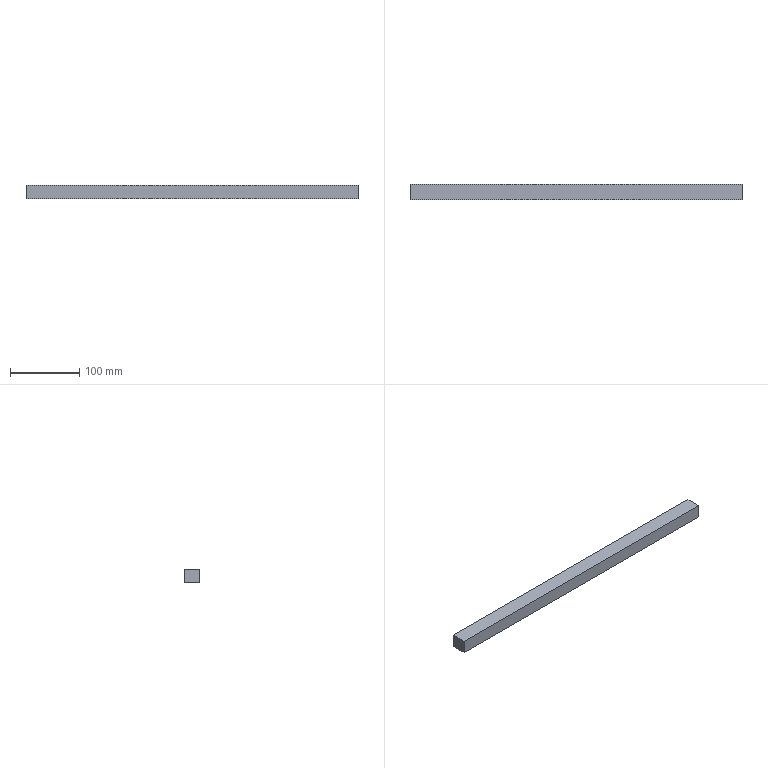Part | SolidWorks | features Extrusion 1 | 1 solid | 6 faces | box 480 x 22 x 20 mm | volume 211200 mm3 | plane 6
STEP:
#1=CARTESIAN_POINT('',(0.,22.,0.));
#2=VERTEX_POINT('',#1);
#3=CARTESIAN_POINT('',(0.,0.,0.));
#4=VERTEX_POINT('',#3);
#5=CARTESIAN_POINT('',(0.,0.,0.));
#6=DIRECTION('',(0.,-1.,0.));
#7=VECTOR('',#6,1000.);
#8=LINE('',#5,#7);
#9=EDGE_CURVE('',#2,#4,#8,.T.);
#10=ORIENTED_EDGE('',*,*,#9,.T.);
#11=CARTESIAN_POINT('',(0.,0.,20.));
#12=VERTEX_POINT('',#11);
#13=CARTESIAN_POINT('',(0.,0.,20.));
#14=DIRECTION('',(0.,0.,-1.));
#15=VECTOR('',#14,1000.);
#16=LINE('',#13,#15);
#17=EDGE_CURVE('',#12,#4,#16,.T.);
#18=ORIENTED_EDGE('',*,*,#17,.F.);
#19=CARTESIAN_POINT('',(0.,22.,20.));
#20=VERTEX_POINT('',#19);
#21=CARTESIAN_POINT('',(0.,0.,20.));
#22=DIRECTION('',(0.,-1.,0.));
#23=VECTOR('',#22,1000.);
#24=LINE('',#21,#23);
#25=EDGE_CURVE('',#20,#12,#24,.T.);
#26=ORIENTED_EDGE('',*,*,#25,.F.);
#27=CARTESIAN_POINT('',(0.,22.,20.));
#28=DIRECTION('',(0.,0.,-1.));
#29=VECTOR('',#28,1000.);
#30=LINE('',#27,#29);
#31=EDGE_CURVE('',#20,#2,#30,.T.);
#32=ORIENTED_EDGE('',*,*,#31,.T.);
#33=EDGE_LOOP('',(#10,#18,#26,#32));
#34=FACE_OUTER_BOUND('',#33,.T.);
#35=CARTESIAN_POINT('',(0.,0.,20.));
#36=DIRECTION('',(1.,0.,0.));
#37=DIRECTION('',(0.,0.,-1.));
#38=AXIS2_PLACEMENT_3D('',#35,#36,#37);
#39=PLANE('',#38);
#40=ADVANCED_FACE('',(#34),#39,.F.);
#41=CARTESIAN_POINT('',(480.,0.,0.));
#42=VERTEX_POINT('',#41);
#43=CARTESIAN_POINT('',(0.,0.,0.));
#44=DIRECTION('',(1.,0.,0.));
#45=VECTOR('',#44,1000.);
#46=LINE('',#43,#45);
#47=EDGE_CURVE('',#4,#42,#46,.T.);
#48=ORIENTED_EDGE('',*,*,#47,.T.);
#49=CARTESIAN_POINT('',(480.,0.,20.));
#50=VERTEX_POINT('',#49);
#51=CARTESIAN_POINT('',(480.,0.,20.));
#52=DIRECTION('',(0.,0.,-1.));
#53=VECTOR('',#52,1000.);
#54=LINE('',#51,#53);
#55=EDGE_CURVE('',#50,#42,#54,.T.);
#56=ORIENTED_EDGE('',*,*,#55,.F.);
#57=CARTESIAN_POINT('',(0.,0.,20.));
#58=DIRECTION('',(1.,0.,0.));
#59=VECTOR('',#58,1000.);
#60=LINE('',#57,#59);
#61=EDGE_CURVE('',#12,#50,#60,.T.);
#62=ORIENTED_EDGE('',*,*,#61,.F.);
#63=ORIENTED_EDGE('',*,*,#17,.T.);
#64=EDGE_LOOP('',(#48,#56,#62,#63));
#65=FACE_OUTER_BOUND('',#64,.T.);
#66=CARTESIAN_POINT('',(0.,0.,20.));
#67=DIRECTION('',(0.,1.,0.));
#68=DIRECTION('',(0.,0.,1.));
#69=AXIS2_PLACEMENT_3D('',#66,#67,#68);
#70=PLANE('',#69);
#71=ADVANCED_FACE('',(#65),#70,.F.);
#72=CARTESIAN_POINT('',(480.,22.,0.));
#73=VERTEX_POINT('',#72);
#74=CARTESIAN_POINT('',(480.,0.,0.));
#75=DIRECTION('',(0.,1.,0.));
#76=VECTOR('',#75,1000.);
#77=LINE('',#74,#76);
#78=EDGE_CURVE('',#42,#73,#77,.T.);
#79=ORIENTED_EDGE('',*,*,#78,.T.);
#80=CARTESIAN_POINT('',(480.,22.,20.));
#81=VERTEX_POINT('',#80);
#82=CARTESIAN_POINT('',(480.,22.,20.));
#83=DIRECTION('',(0.,0.,-1.));
#84=VECTOR('',#83,1000.);
#85=LINE('',#82,#84);
#86=EDGE_CURVE('',#81,#73,#85,.T.);
#87=ORIENTED_EDGE('',*,*,#86,.F.);
#88=CARTESIAN_POINT('',(480.,0.,20.));
#89=DIRECTION('',(0.,1.,0.));
#90=VECTOR('',#89,1000.);
#91=LINE('',#88,#90);
#92=EDGE_CURVE('',#50,#81,#91,.T.);
#93=ORIENTED_EDGE('',*,*,#92,.F.);
#94=ORIENTED_EDGE('',*,*,#55,.T.);
#95=EDGE_LOOP('',(#79,#87,#93,#94));
#96=FACE_OUTER_BOUND('',#95,.T.);
#97=CARTESIAN_POINT('',(480.,0.,20.));
#98=DIRECTION('',(-1.,0.,0.));
#99=DIRECTION('',(0.,0.,1.));
#100=AXIS2_PLACEMENT_3D('',#97,#98,#99);
#101=PLANE('',#100);
#102=ADVANCED_FACE('',(#96),#101,.F.);
#103=CARTESIAN_POINT('',(0.,22.,0.));
#104=DIRECTION('',(-1.,0.,0.));
#105=VECTOR('',#104,1000.);
#106=LINE('',#103,#105);
#107=EDGE_CURVE('',#73,#2,#106,.T.);
#108=ORIENTED_EDGE('',*,*,#107,.T.);
#109=ORIENTED_EDGE('',*,*,#31,.F.);
#110=CARTESIAN_POINT('',(0.,22.,20.));
#111=DIRECTION('',(-1.,0.,0.));
#112=VECTOR('',#111,1000.);
#113=LINE('',#110,#112);
#114=EDGE_CURVE('',#81,#20,#113,.T.);
#115=ORIENTED_EDGE('',*,*,#114,.F.);
#116=ORIENTED_EDGE('',*,*,#86,.T.);
#117=EDGE_LOOP('',(#108,#109,#115,#116));
#118=FACE_OUTER_BOUND('',#117,.T.);
#119=CARTESIAN_POINT('',(0.,22.,20.));
#120=DIRECTION('',(0.,-1.,0.));
#121=DIRECTION('',(0.,0.,-1.));
#122=AXIS2_PLACEMENT_3D('',#119,#120,#121);
#123=PLANE('',#122);
#124=ADVANCED_FACE('',(#118),#123,.F.);
#125=ORIENTED_EDGE('',*,*,#25,.T.);
#126=ORIENTED_EDGE('',*,*,#61,.T.);
#127=ORIENTED_EDGE('',*,*,#92,.T.);
#128=ORIENTED_EDGE('',*,*,#114,.T.);
#129=EDGE_LOOP('',(#125,#126,#127,#128));
#130=FACE_OUTER_BOUND('',#129,.T.);
#131=CARTESIAN_POINT('',(0.,0.,20.));
#132=DIRECTION('',(0.,0.,-1.));
#133=DIRECTION('',(-1.,0.,0.));
#134=AXIS2_PLACEMENT_3D('',#131,#132,#133);
#135=PLANE('',#134);
#136=ADVANCED_FACE('',(#130),#135,.F.);
#137=ORIENTED_EDGE('',*,*,#9,.F.);
#138=ORIENTED_EDGE('',*,*,#107,.F.);
#139=ORIENTED_EDGE('',*,*,#78,.F.);
#140=ORIENTED_EDGE('',*,*,#47,.F.);
#141=EDGE_LOOP('',(#137,#138,#139,#140));
#142=FACE_OUTER_BOUND('',#141,.T.);
#143=CARTESIAN_POINT('',(0.,0.,0.));
#144=DIRECTION('',(0.,0.,-1.));
#145=DIRECTION('',(-1.,0.,0.));
#146=AXIS2_PLACEMENT_3D('',#143,#144,#145);
#147=PLANE('',#146);
#148=ADVANCED_FACE('',(#142),#147,.T.);
#149=CLOSED_SHELL('',(#40,#71,#102,#124,#136,#148));
#150=MANIFOLD_SOLID_BREP('',#149);
#151=CARTESIAN_POINT('',(0.,0.,0.));
#152=DIRECTION('',(0.,0.,1.));
#153=DIRECTION('',(1.,0.,0.));
#154=AXIS2_PLACEMENT_3D('',#151,#152,#153);
#155=(LENGTH_UNIT()NAMED_UNIT(*)SI_UNIT(.MILLI.,.METRE.));
#156=UNCERTAINTY_MEASURE_WITH_UNIT(LENGTH_MEASURE(0.00001),#155,'','');
#157=(NAMED_UNIT(*)PLANE_ANGLE_UNIT()SI_UNIT($,.RADIAN.));
#158=(NAMED_UNIT(*)SI_UNIT($,.STERADIAN.)SOLID_ANGLE_UNIT());
#159=(GEOMETRIC_REPRESENTATION_CONTEXT(3)GLOBAL_UNCERTAINTY_ASSIGNED_CONTEXT((#156))GLOBAL_UNIT_ASSIGNED_CONTEXT((#155,#157,#158))REPRESENTATION_CONTEXT('',''));
#160=ADVANCED_BREP_SHAPE_REPRESENTATION('',(#150,#154),#159);